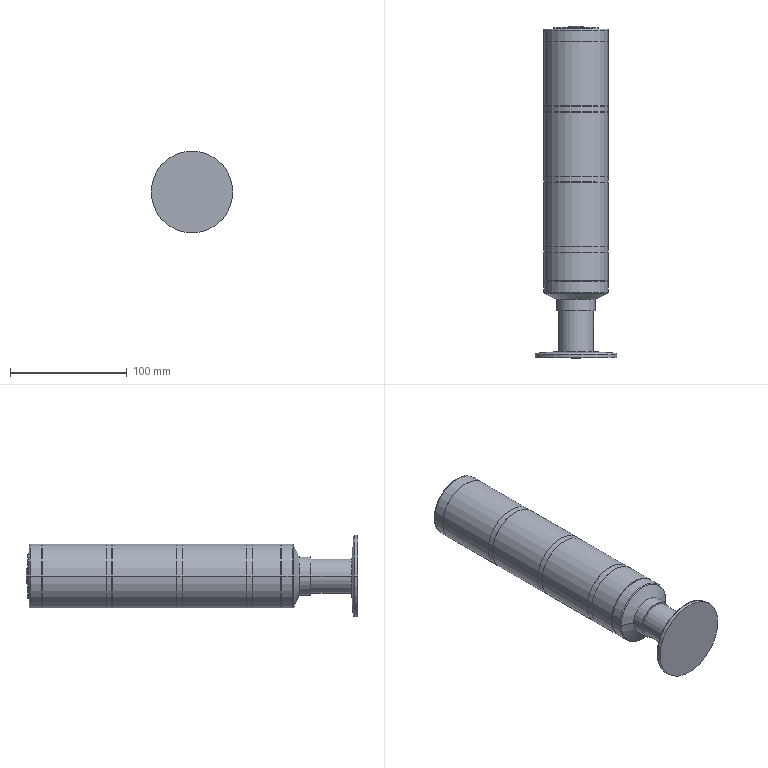Part | NX | features BREP 11 | 11 solids | 89 faces | box 70 x 284.2 x 70 mm | volume 574095 mm3 | cylinder 48 | plane 27 | torus 10 | cone 4 | commonest cylinder face diameters 55 x18 22.355 x6 47.695 x6 49 x6 12.176 x2 29.984 x2